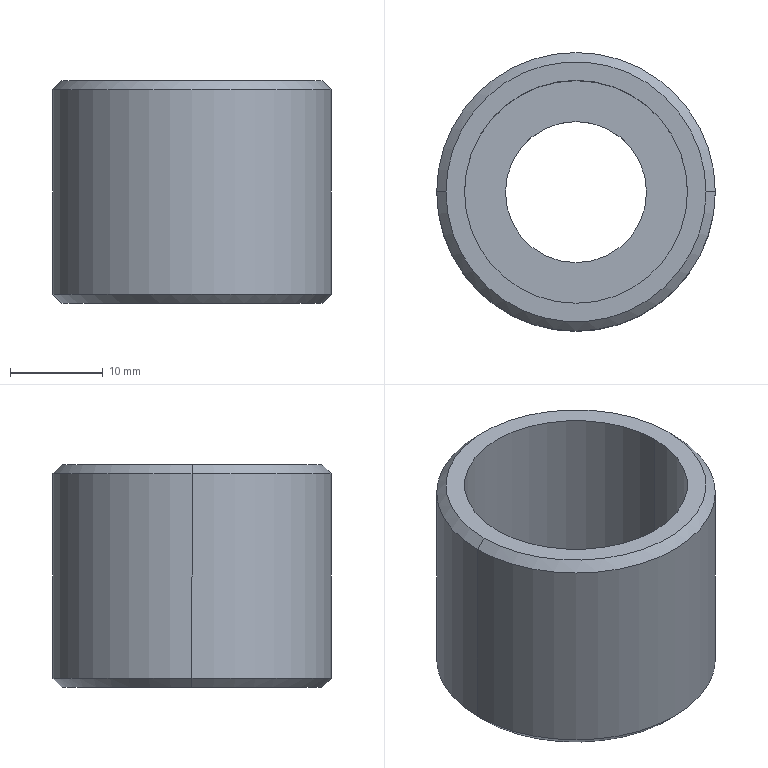Part | STEP file | fBY02F02M-00-16A | 1 solid | 16 faces | box 30 x 30 x 24 mm | volume 7122 mm3 | cylinder 8 | cone 4 | plane 4 | commonest cylinder face diameters 15.2 x2 21 x2 24 x2 30 x2
STEP:
#1=CARTESIAN_POINT('',(0.,0.,0.));
#2=DIRECTION('',(0.,0.,1.));
#3=DIRECTION('',(1.,0.,0.));
#4=AXIS2_PLACEMENT_3D('',#1,#2,#3);
#5=CARTESIAN_POINT('',(-15.,0.,23.));
#6=VERTEX_POINT('',#5);
#7=CARTESIAN_POINT('',(15.,0.,23.));
#8=VERTEX_POINT('',#7);
#9=CARTESIAN_POINT('',(0.,0.,23.));
#10=DIRECTION('',(0.,0.,-1.));
#11=DIRECTION('',(-1.,0.,0.));
#12=AXIS2_PLACEMENT_3D('',#9,#10,#11);
#13=CIRCLE('',#12,15.);
#14=CARTESIAN_POINT('',(0.,0.,24.));
#15=DIRECTION('',(0.,0.,-1.));
#16=DIRECTION('',(-1.,0.,0.));
#17=AXIS2_PLACEMENT_3D('',#14,#15,#16);
#18=CYLINDRICAL_SURFACE('',#17,15.);
#19=CARTESIAN_POINT('',(0.,1.));
#20=DIRECTION('',(1.,0.));
#21=VECTOR('',#20,1.);
#22=LINE('',#19,#21);
#23=(GEOMETRIC_REPRESENTATION_CONTEXT(2)PARAMETRIC_REPRESENTATION_CONTEXT()REPRESENTATION_CONTEXT('',''));
#24=DEFINITIONAL_REPRESENTATION('',(#22),#23);
#25=PCURVE('',#18,#24);
#26=CARTESIAN_POINT('',(0.,0.,23.));
#27=DIRECTION('',(0.,0.,-1.));
#28=DIRECTION('',(-1.,0.,0.));
#29=AXIS2_PLACEMENT_3D('',#26,#27,#28);
#30=CONICAL_SURFACE('',#29,15.,0.7854);
#31=CARTESIAN_POINT('',(0.,0.));
#32=DIRECTION('',(1.,0.));
#33=VECTOR('',#32,1.);
#34=LINE('',#31,#33);
#35=(GEOMETRIC_REPRESENTATION_CONTEXT(2)PARAMETRIC_REPRESENTATION_CONTEXT()REPRESENTATION_CONTEXT('',''));
#36=DEFINITIONAL_REPRESENTATION('',(#34),#35);
#37=PCURVE('',#30,#36);
#38=SURFACE_CURVE('',#13,(#25,#37),.PCURVE_S1.);
#39=EDGE_CURVE('',#6,#8,#38,.T.);
#40=ORIENTED_EDGE('',*,*,#39,.T.);
#41=CARTESIAN_POINT('',(15.,0.,1.));
#42=VERTEX_POINT('',#41);
#43=CARTESIAN_POINT('',(15.,0.,24.));
#44=DIRECTION('',(0.,0.,-1.));
#45=VECTOR('',#44,1.);
#46=LINE('',#43,#45);
#47=CARTESIAN_POINT('',(3.142,0.));
#48=DIRECTION('',(0.,1.));
#49=VECTOR('',#48,1.);
#50=LINE('',#47,#49);
#51=(GEOMETRIC_REPRESENTATION_CONTEXT(2)PARAMETRIC_REPRESENTATION_CONTEXT()REPRESENTATION_CONTEXT('',''));
#52=DEFINITIONAL_REPRESENTATION('',(#50),#51);
#53=PCURVE('',#18,#52);
#54=CARTESIAN_POINT('',(0.,0.,24.));
#55=DIRECTION('',(0.,0.,-1.));
#56=DIRECTION('',(-1.,0.,0.));
#57=AXIS2_PLACEMENT_3D('',#54,#55,#56);
#58=CYLINDRICAL_SURFACE('',#57,15.);
#59=CARTESIAN_POINT('',(3.142,0.));
#60=DIRECTION('',(0.,1.));
#61=VECTOR('',#60,1.);
#62=LINE('',#59,#61);
#63=(GEOMETRIC_REPRESENTATION_CONTEXT(2)PARAMETRIC_REPRESENTATION_CONTEXT()REPRESENTATION_CONTEXT('',''));
#64=DEFINITIONAL_REPRESENTATION('',(#62),#63);
#65=PCURVE('',#58,#64);
#66=SURFACE_CURVE('',#46,(#53,#65),.PCURVE_S1.);
#67=EDGE_CURVE('',#8,#42,#66,.T.);
#68=ORIENTED_EDGE('',*,*,#67,.T.);
#69=CARTESIAN_POINT('',(-15.,0.,1.));
#70=VERTEX_POINT('',#69);
#71=CARTESIAN_POINT('',(0.,0.,1.));
#72=DIRECTION('',(0.,0.,1.));
#73=DIRECTION('',(-1.,0.,0.));
#74=AXIS2_PLACEMENT_3D('',#71,#72,#73);
#75=CIRCLE('',#74,15.);
#76=CARTESIAN_POINT('',(6.283,23.));
#77=DIRECTION('',(-1.,0.));
#78=VECTOR('',#77,1.);
#79=LINE('',#76,#78);
#80=(GEOMETRIC_REPRESENTATION_CONTEXT(2)PARAMETRIC_REPRESENTATION_CONTEXT()REPRESENTATION_CONTEXT('',''));
#81=DEFINITIONAL_REPRESENTATION('',(#79),#80);
#82=PCURVE('',#18,#81);
#83=CARTESIAN_POINT('',(0.,0.,1.));
#84=DIRECTION('',(0.,0.,1.));
#85=DIRECTION('',(1.,0.,0.));
#86=AXIS2_PLACEMENT_3D('',#83,#84,#85);
#87=CONICAL_SURFACE('',#86,15.,0.7854);
#88=CARTESIAN_POINT('',(-3.142,0.));
#89=DIRECTION('',(1.,0.));
#90=VECTOR('',#89,1.);
#91=LINE('',#88,#90);
#92=(GEOMETRIC_REPRESENTATION_CONTEXT(2)PARAMETRIC_REPRESENTATION_CONTEXT()REPRESENTATION_CONTEXT('',''));
#93=DEFINITIONAL_REPRESENTATION('',(#91),#92);
#94=PCURVE('',#87,#93);
#95=SURFACE_CURVE('',#75,(#82,#94),.PCURVE_S1.);
#96=EDGE_CURVE('',#42,#70,#95,.T.);
#97=ORIENTED_EDGE('',*,*,#96,.T.);
#98=CARTESIAN_POINT('',(-15.,0.,24.));
#99=DIRECTION('',(0.,0.,-1.));
#100=VECTOR('',#99,1.);
#101=LINE('',#98,#100);
#102=CARTESIAN_POINT('',(0.,0.));
#103=DIRECTION('',(0.,1.));
#104=VECTOR('',#103,1.);
#105=LINE('',#102,#104);
#106=(GEOMETRIC_REPRESENTATION_CONTEXT(2)PARAMETRIC_REPRESENTATION_CONTEXT()REPRESENTATION_CONTEXT('',''));
#107=DEFINITIONAL_REPRESENTATION('',(#105),#106);
#108=PCURVE('',#18,#107);
#109=CARTESIAN_POINT('',(6.283,0.));
#110=DIRECTION('',(0.,1.));
#111=VECTOR('',#110,1.);
#112=LINE('',#109,#111);
#113=(GEOMETRIC_REPRESENTATION_CONTEXT(2)PARAMETRIC_REPRESENTATION_CONTEXT()REPRESENTATION_CONTEXT('',''));
#114=DEFINITIONAL_REPRESENTATION('',(#112),#113);
#115=PCURVE('',#58,#114);
#116=SURFACE_CURVE('',#101,(#108,#115),.PCURVE_S1.);
#117=EDGE_CURVE('',#6,#70,#116,.T.);
#118=ORIENTED_EDGE('',*,*,#117,.F.);
#119=EDGE_LOOP('',(#40,#68,#97,#118));
#120=FACE_BOUND('',#119,.T.);
#121=ADVANCED_FACE('',(#120),#18,.T.);
#122=CARTESIAN_POINT('',(14.,0.,0.));
#123=VERTEX_POINT('',#122);
#124=CARTESIAN_POINT('',(-14.,0.,0.));
#125=VERTEX_POINT('',#124);
#126=CARTESIAN_POINT('',(0.,0.,0.));
#127=DIRECTION('',(0.,0.,1.));
#128=DIRECTION('',(1.,0.,0.));
#129=AXIS2_PLACEMENT_3D('',#126,#127,#128);
#130=CIRCLE('',#129,14.);
#131=CARTESIAN_POINT('',(0.,-1.));
#132=DIRECTION('',(1.,0.));
#133=VECTOR('',#132,1.);
#134=LINE('',#131,#133);
#135=(GEOMETRIC_REPRESENTATION_CONTEXT(2)PARAMETRIC_REPRESENTATION_CONTEXT()REPRESENTATION_CONTEXT('',''));
#136=DEFINITIONAL_REPRESENTATION('',(#134),#135);
#137=PCURVE('',#87,#136);
#138=CARTESIAN_POINT('',(0.,0.,0.));
#139=DIRECTION('',(0.,0.,1.));
#140=DIRECTION('',(1.,0.,0.));
#141=AXIS2_PLACEMENT_3D('',#138,#139,#140);
#142=PLANE('',#141);
#143=CARTESIAN_POINT('',(0.,0.));
#144=DIRECTION('',(1.,0.));
#145=AXIS2_PLACEMENT_2D('',#143,#144);
#146=CIRCLE('',#145,14.);
#147=(GEOMETRIC_REPRESENTATION_CONTEXT(2)PARAMETRIC_REPRESENTATION_CONTEXT()REPRESENTATION_CONTEXT('',''));
#148=DEFINITIONAL_REPRESENTATION('',(#146),#147);
#149=PCURVE('',#142,#148);
#150=SURFACE_CURVE('',#130,(#137,#149),.PCURVE_S1.);
#151=EDGE_CURVE('',#123,#125,#150,.T.);
#152=ORIENTED_EDGE('',*,*,#151,.T.);
#153=CARTESIAN_POINT('',(-15.,0.,1.));
#154=DIRECTION('',(-0.7071,0.,0.7071));
#155=VECTOR('',#154,1.);
#156=LINE('',#153,#155);
#157=CARTESIAN_POINT('',(3.142,0.));
#158=DIRECTION('',(0.,1.));
#159=VECTOR('',#158,1.);
#160=LINE('',#157,#159);
#161=(GEOMETRIC_REPRESENTATION_CONTEXT(2)PARAMETRIC_REPRESENTATION_CONTEXT()REPRESENTATION_CONTEXT('',''));
#162=DEFINITIONAL_REPRESENTATION('',(#160),#161);
#163=PCURVE('',#87,#162);
#164=CARTESIAN_POINT('',(0.,0.,1.));
#165=DIRECTION('',(0.,0.,1.));
#166=DIRECTION('',(1.,0.,0.));
#167=AXIS2_PLACEMENT_3D('',#164,#165,#166);
#168=CONICAL_SURFACE('',#167,15.,0.7854);
#169=CARTESIAN_POINT('',(3.142,0.));
#170=DIRECTION('',(0.,1.));
#171=VECTOR('',#170,1.);
#172=LINE('',#169,#171);
#173=(GEOMETRIC_REPRESENTATION_CONTEXT(2)PARAMETRIC_REPRESENTATION_CONTEXT()REPRESENTATION_CONTEXT('',''));
#174=DEFINITIONAL_REPRESENTATION('',(#172),#173);
#175=PCURVE('',#168,#174);
#176=SURFACE_CURVE('',#156,(#163,#175),.PCURVE_S1.);
#177=EDGE_CURVE('',#125,#70,#176,.T.);
#178=ORIENTED_EDGE('',*,*,#177,.T.);
#179=ORIENTED_EDGE('',*,*,#96,.F.);
#180=CARTESIAN_POINT('',(15.,0.,1.));
#181=DIRECTION('',(0.7071,0.,0.7071));
#182=VECTOR('',#181,1.);
#183=LINE('',#180,#182);
#184=CARTESIAN_POINT('',(0.,0.));
#185=DIRECTION('',(0.,1.));
#186=VECTOR('',#185,1.);
#187=LINE('',#184,#186);
#188=(GEOMETRIC_REPRESENTATION_CONTEXT(2)PARAMETRIC_REPRESENTATION_CONTEXT()REPRESENTATION_CONTEXT('',''));
#189=DEFINITIONAL_REPRESENTATION('',(#187),#188);
#190=PCURVE('',#87,#189);
#191=CARTESIAN_POINT('',(6.283,0.));
#192=DIRECTION('',(0.,1.));
#193=VECTOR('',#192,1.);
#194=LINE('',#191,#193);
#195=(GEOMETRIC_REPRESENTATION_CONTEXT(2)PARAMETRIC_REPRESENTATION_CONTEXT()REPRESENTATION_CONTEXT('',''));
#196=DEFINITIONAL_REPRESENTATION('',(#194),#195);
#197=PCURVE('',#168,#196);
#198=SURFACE_CURVE('',#183,(#190,#197),.PCURVE_S1.);
#199=EDGE_CURVE('',#123,#42,#198,.T.);
#200=ORIENTED_EDGE('',*,*,#199,.F.);
#201=EDGE_LOOP('',(#152,#178,#179,#200));
#202=FACE_BOUND('',#201,.T.);
#203=ADVANCED_FACE('',(#202),#87,.T.);
#204=CARTESIAN_POINT('',(-14.,0.,24.));
#205=VERTEX_POINT('',#204);
#206=CARTESIAN_POINT('',(14.,0.,24.));
#207=VERTEX_POINT('',#206);
#208=CARTESIAN_POINT('',(0.,0.,24.));
#209=DIRECTION('',(0.,0.,-1.));
#210=DIRECTION('',(-1.,0.,0.));
#211=AXIS2_PLACEMENT_3D('',#208,#209,#210);
#212=CIRCLE('',#211,14.);
#213=CARTESIAN_POINT('',(0.,-1.));
#214=DIRECTION('',(1.,0.));
#215=VECTOR('',#214,1.);
#216=LINE('',#213,#215);
#217=(GEOMETRIC_REPRESENTATION_CONTEXT(2)PARAMETRIC_REPRESENTATION_CONTEXT()REPRESENTATION_CONTEXT('',''));
#218=DEFINITIONAL_REPRESENTATION('',(#216),#217);
#219=PCURVE('',#30,#218);
#220=CARTESIAN_POINT('',(0.,0.,24.));
#221=DIRECTION('',(0.,0.,1.));
#222=DIRECTION('',(1.,0.,0.));
#223=AXIS2_PLACEMENT_3D('',#220,#221,#222);
#224=PLANE('',#223);
#225=CARTESIAN_POINT('',(-14.,0.));
#226=CARTESIAN_POINT('',(-14.,24.249));
#227=CARTESIAN_POINT('',(7.,12.124));
#228=CARTESIAN_POINT('',(28.,0.));
#229=CARTESIAN_POINT('',(7.,-12.124));
#230=CARTESIAN_POINT('',(-14.,-24.249));
#231=CARTESIAN_POINT('',(-14.,0.));
#232=(BOUNDED_CURVE()B_SPLINE_CURVE(2,(#225,#226,#227,#228,#229,#230,#231),.UNSPECIFIED.,.T.,.F.)B_SPLINE_CURVE_WITH_KNOTS((1,2,2,2,2,1),(-2.094,0.,2.094,4.189,6.283,8.378),.UNSPECIFIED.)CURVE()GEOMETRIC_REPRESENTATION_ITEM()RATIONAL_B_SPLINE_CURVE((1.,0.5,1.,0.5,1.,0.5,1.))REPRESENTATION_ITEM(''));
#233=(GEOMETRIC_REPRESENTATION_CONTEXT(2)PARAMETRIC_REPRESENTATION_CONTEXT()REPRESENTATION_CONTEXT('',''));
#234=DEFINITIONAL_REPRESENTATION('',(#232),#233);
#235=PCURVE('',#224,#234);
#236=SURFACE_CURVE('',#212,(#219,#235),.PCURVE_S1.);
#237=EDGE_CURVE('',#205,#207,#236,.T.);
#238=ORIENTED_EDGE('',*,*,#237,.T.);
#239=CARTESIAN_POINT('',(15.,0.,23.));
#240=DIRECTION('',(0.7071,0.,-0.7071));
#241=VECTOR('',#240,1.);
#242=LINE('',#239,#241);
#243=CARTESIAN_POINT('',(3.142,0.));
#244=DIRECTION('',(0.,1.));
#245=VECTOR('',#244,1.);
#246=LINE('',#243,#245);
#247=(GEOMETRIC_REPRESENTATION_CONTEXT(2)PARAMETRIC_REPRESENTATION_CONTEXT()REPRESENTATION_CONTEXT('',''));
#248=DEFINITIONAL_REPRESENTATION('',(#246),#247);
#249=PCURVE('',#30,#248);
#250=CARTESIAN_POINT('',(0.,0.,23.));
#251=DIRECTION('',(0.,0.,-1.));
#252=DIRECTION('',(-1.,0.,0.));
#253=AXIS2_PLACEMENT_3D('',#250,#251,#252);
#254=CONICAL_SURFACE('',#253,15.,0.7854);
#255=CARTESIAN_POINT('',(3.142,0.));
#256=DIRECTION('',(0.,1.));
#257=VECTOR('',#256,1.);
#258=LINE('',#255,#257);
#259=(GEOMETRIC_REPRESENTATION_CONTEXT(2)PARAMETRIC_REPRESENTATION_CONTEXT()REPRESENTATION_CONTEXT('',''));
#260=DEFINITIONAL_REPRESENTATION('',(#258),#259);
#261=PCURVE('',#254,#260);
#262=SURFACE_CURVE('',#242,(#249,#261),.PCURVE_S1.);
#263=EDGE_CURVE('',#207,#8,#262,.T.);
#264=ORIENTED_EDGE('',*,*,#263,.T.);
#265=ORIENTED_EDGE('',*,*,#39,.F.);
#266=CARTESIAN_POINT('',(-15.,0.,23.));
#267=DIRECTION('',(-0.7071,0.,-0.7071));
#268=VECTOR('',#267,1.);
#269=LINE('',#266,#268);
#270=CARTESIAN_POINT('',(0.,0.));
#271=DIRECTION('',(0.,1.));
#272=VECTOR('',#271,1.);
#273=LINE('',#270,#272);
#274=(GEOMETRIC_REPRESENTATION_CONTEXT(2)PARAMETRIC_REPRESENTATION_CONTEXT()REPRESENTATION_CONTEXT('',''));
#275=DEFINITIONAL_REPRESENTATION('',(#273),#274);
#276=PCURVE('',#30,#275);
#277=CARTESIAN_POINT('',(6.283,0.));
#278=DIRECTION('',(0.,1.));
#279=VECTOR('',#278,1.);
#280=LINE('',#277,#279);
#281=(GEOMETRIC_REPRESENTATION_CONTEXT(2)PARAMETRIC_REPRESENTATION_CONTEXT()REPRESENTATION_CONTEXT('',''));
#282=DEFINITIONAL_REPRESENTATION('',(#280),#281);
#283=PCURVE('',#254,#282);
#284=SURFACE_CURVE('',#269,(#276,#283),.PCURVE_S1.);
#285=EDGE_CURVE('',#205,#6,#284,.T.);
#286=ORIENTED_EDGE('',*,*,#285,.F.);
#287=EDGE_LOOP('',(#238,#264,#265,#286));
#288=FACE_BOUND('',#287,.T.);
#289=ADVANCED_FACE('',(#288),#30,.T.);
#290=CARTESIAN_POINT('',(-10.5,0.,1.5));
#291=VERTEX_POINT('',#290);
#292=CARTESIAN_POINT('',(-10.5,0.,0.));
#293=VERTEX_POINT('',#292);
#294=CARTESIAN_POINT('',(-10.5,0.,1.5));
#295=DIRECTION('',(0.,0.,-1.));
#296=VECTOR('',#295,1.);
#297=LINE('',#294,#296);
#298=CARTESIAN_POINT('',(0.,0.,1.5));
#299=DIRECTION('',(0.,0.,-1.));
#300=DIRECTION('',(-1.,0.,0.));
#301=AXIS2_PLACEMENT_3D('',#298,#299,#300);
#302=CYLINDRICAL_SURFACE('',#301,10.5);
#303=CARTESIAN_POINT('',(6.283,0.));
#304=DIRECTION('',(0.,1.));
#305=VECTOR('',#304,1.);
#306=LINE('',#303,#305);
#307=(GEOMETRIC_REPRESENTATION_CONTEXT(2)PARAMETRIC_REPRESENTATION_CONTEXT()REPRESENTATION_CONTEXT('',''));
#308=DEFINITIONAL_REPRESENTATION('',(#306),#307);
#309=PCURVE('',#302,#308);
#310=CARTESIAN_POINT('',(0.,0.,1.5));
#311=DIRECTION('',(0.,0.,-1.));
#312=DIRECTION('',(-1.,0.,0.));
#313=AXIS2_PLACEMENT_3D('',#310,#311,#312);
#314=CYLINDRICAL_SURFACE('',#313,10.5);
#315=CARTESIAN_POINT('',(0.,0.));
#316=DIRECTION('',(0.,1.));
#317=VECTOR('',#316,1.);
#318=LINE('',#315,#317);
#319=(GEOMETRIC_REPRESENTATION_CONTEXT(2)PARAMETRIC_REPRESENTATION_CONTEXT()REPRESENTATION_CONTEXT('',''));
#320=DEFINITIONAL_REPRESENTATION('',(#318),#319);
#321=PCURVE('',#314,#320);
#322=SURFACE_CURVE('',#297,(#309,#321),.PCURVE_S1.);
#323=EDGE_CURVE('',#291,#293,#322,.T.);
#324=ORIENTED_EDGE('',*,*,#323,.T.);
#325=CARTESIAN_POINT('',(10.5,0.,0.));
#326=VERTEX_POINT('',#325);
#327=CARTESIAN_POINT('',(0.,0.,0.));
#328=DIRECTION('',(0.,0.,-1.));
#329=DIRECTION('',(-1.,0.,0.));
#330=AXIS2_PLACEMENT_3D('',#327,#328,#329);
#331=CIRCLE('',#330,10.5);
#332=CARTESIAN_POINT('',(0.,1.5));
#333=DIRECTION('',(1.,0.));
#334=VECTOR('',#333,1.);
#335=LINE('',#332,#334);
#336=(GEOMETRIC_REPRESENTATION_CONTEXT(2)PARAMETRIC_REPRESENTATION_CONTEXT()REPRESENTATION_CONTEXT('',''));
#337=DEFINITIONAL_REPRESENTATION('',(#335),#336);
#338=PCURVE('',#302,#337);
#339=CARTESIAN_POINT('',(-10.5,0.));
#340=CARTESIAN_POINT('',(-10.5,18.187));
#341=CARTESIAN_POINT('',(5.25,9.093));
#342=CARTESIAN_POINT('',(21.,0.));
#343=CARTESIAN_POINT('',(5.25,-9.093));
#344=CARTESIAN_POINT('',(-10.5,-18.187));
#345=CARTESIAN_POINT('',(-10.5,0.));
#346=(BOUNDED_CURVE()B_SPLINE_CURVE(2,(#339,#340,#341,#342,#343,#344,#345),.UNSPECIFIED.,.T.,.F.)B_SPLINE_CURVE_WITH_KNOTS((1,2,2,2,2,1),(-2.094,0.,2.094,4.189,6.283,8.378),.UNSPECIFIED.)CURVE()GEOMETRIC_REPRESENTATION_ITEM()RATIONAL_B_SPLINE_CURVE((1.,0.5,1.,0.5,1.,0.5,1.))REPRESENTATION_ITEM(''));
#347=(GEOMETRIC_REPRESENTATION_CONTEXT(2)PARAMETRIC_REPRESENTATION_CONTEXT()REPRESENTATION_CONTEXT('',''));
#348=DEFINITIONAL_REPRESENTATION('',(#346),#347);
#349=PCURVE('',#142,#348);
#350=SURFACE_CURVE('',#331,(#338,#349),.PCURVE_S1.);
#351=EDGE_CURVE('',#326,#293,#350,.T.);
#352=ORIENTED_EDGE('',*,*,#351,.F.);
#353=CARTESIAN_POINT('',(10.5,0.,1.5));
#354=VERTEX_POINT('',#353);
#355=CARTESIAN_POINT('',(10.5,0.,1.5));
#356=DIRECTION('',(0.,0.,-1.));
#357=VECTOR('',#356,1.);
#358=LINE('',#355,#357);
#359=CARTESIAN_POINT('',(3.142,0.));
#360=DIRECTION('',(0.,1.));
#361=VECTOR('',#360,1.);
#362=LINE('',#359,#361);
#363=(GEOMETRIC_REPRESENTATION_CONTEXT(2)PARAMETRIC_REPRESENTATION_CONTEXT()REPRESENTATION_CONTEXT('',''));
#364=DEFINITIONAL_REPRESENTATION('',(#362),#363);
#365=PCURVE('',#302,#364);
#366=CARTESIAN_POINT('',(3.142,0.));
#367=DIRECTION('',(0.,1.));
#368=VECTOR('',#367,1.);
#369=LINE('',#366,#368);
#370=(GEOMETRIC_REPRESENTATION_CONTEXT(2)PARAMETRIC_REPRESENTATION_CONTEXT()REPRESENTATION_CONTEXT('',''));
#371=DEFINITIONAL_REPRESENTATION('',(#369),#370);
#372=PCURVE('',#314,#371);
#373=SURFACE_CURVE('',#358,(#365,#372),.PCURVE_S1.);
#374=EDGE_CURVE('',#354,#326,#373,.T.);
#375=ORIENTED_EDGE('',*,*,#374,.F.);
#376=CARTESIAN_POINT('',(0.,0.,1.5));
#377=DIRECTION('',(0.,0.,-1.));
#378=DIRECTION('',(-1.,0.,0.));
#379=AXIS2_PLACEMENT_3D('',#376,#377,#378);
#380=CIRCLE('',#379,10.5);
#381=CARTESIAN_POINT('',(0.,0.));
#382=DIRECTION('',(1.,0.));
#383=VECTOR('',#382,1.);
#384=LINE('',#381,#383);
#385=(GEOMETRIC_REPRESENTATION_CONTEXT(2)PARAMETRIC_REPRESENTATION_CONTEXT()REPRESENTATION_CONTEXT('',''));
#386=DEFINITIONAL_REPRESENTATION('',(#384),#385);
#387=PCURVE('',#302,#386);
#388=CARTESIAN_POINT('',(0.,0.,1.5));
#389=DIRECTION('',(0.,0.,-1.));
#390=DIRECTION('',(-1.,0.,0.));
#391=AXIS2_PLACEMENT_3D('',#388,#389,#390);
#392=PLANE('',#391);
#393=CARTESIAN_POINT('',(0.,0.));
#394=DIRECTION('',(1.,0.));
#395=AXIS2_PLACEMENT_2D('',#393,#394);
#396=CIRCLE('',#395,10.5);
#397=(GEOMETRIC_REPRESENTATION_CONTEXT(2)PARAMETRIC_REPRESENTATION_CONTEXT()REPRESENTATION_CONTEXT('',''));
#398=DEFINITIONAL_REPRESENTATION('',(#396),#397);
#399=PCURVE('',#392,#398);
#400=SURFACE_CURVE('',#380,(#387,#399),.PCURVE_S1.);
#401=EDGE_CURVE('',#354,#291,#400,.T.);
#402=ORIENTED_EDGE('',*,*,#401,.T.);
#403=EDGE_LOOP('',(#324,#352,#375,#402));
#404=FACE_BOUND('',#403,.F.);
#405=ADVANCED_FACE('',(#404),#302,.F.);
#406=CARTESIAN_POINT('',(12.,0.,5.));
#407=VERTEX_POINT('',#406);
#408=CARTESIAN_POINT('',(12.,0.,24.));
#409=VERTEX_POINT('',#408);
#410=CARTESIAN_POINT('',(12.,0.,5.));
#411=DIRECTION('',(0.,0.,1.));
#412=VECTOR('',#411,1.);
#413=LINE('',#410,#412);
#414=CARTESIAN_POINT('',(0.,0.,5.));
#415=DIRECTION('',(0.,0.,1.));
#416=DIRECTION('',(1.,0.,0.));
#417=AXIS2_PLACEMENT_3D('',#414,#415,#416);
#418=CYLINDRICAL_SURFACE('',#417,12.);
#419=CARTESIAN_POINT('',(6.283,0.));
#420=DIRECTION('',(0.,1.));
#421=VECTOR('',#420,1.);
#422=LINE('',#419,#421);
#423=(GEOMETRIC_REPRESENTATION_CONTEXT(2)PARAMETRIC_REPRESENTATION_CONTEXT()REPRESENTATION_CONTEXT('',''));
#424=DEFINITIONAL_REPRESENTATION('',(#422),#423);
#425=PCURVE('',#418,#424);
#426=CARTESIAN_POINT('',(0.,0.,5.));
#427=DIRECTION('',(0.,0.,1.));
#428=DIRECTION('',(1.,0.,0.));
#429=AXIS2_PLACEMENT_3D('',#426,#427,#428);
#430=CYLINDRICAL_SURFACE('',#429,12.);
#431=CARTESIAN_POINT('',(0.,0.));
#432=DIRECTION('',(0.,1.));
#433=VECTOR('',#432,1.);
#434=LINE('',#431,#433);
#435=(GEOMETRIC_REPRESENTATION_CONTEXT(2)PARAMETRIC_REPRESENTATION_CONTEXT()REPRESENTATION_CONTEXT('',''));
#436=DEFINITIONAL_REPRESENTATION('',(#434),#435);
#437=PCURVE('',#430,#436);
#438=SURFACE_CURVE('',#413,(#425,#437),.PCURVE_S1.);
#439=EDGE_CURVE('',#407,#409,#438,.T.);
#440=ORIENTED_EDGE('',*,*,#439,.T.);
#441=CARTESIAN_POINT('',(-12.,0.,24.));
#442=VERTEX_POINT('',#441);
#443=CARTESIAN_POINT('',(0.,0.,24.));
#444=DIRECTION('',(0.,0.,-1.));
#445=DIRECTION('',(1.,0.,0.));
#446=AXIS2_PLACEMENT_3D('',#443,#444,#445);
#447=CIRCLE('',#446,12.);
#448=CARTESIAN_POINT('',(6.283,19.));
#449=DIRECTION('',(-1.,0.));
#450=VECTOR('',#449,1.);
#451=LINE('',#448,#450);
#452=(GEOMETRIC_REPRESENTATION_CONTEXT(2)PARAMETRIC_REPRESENTATION_CONTEXT()REPRESENTATION_CONTEXT('',''));
#453=DEFINITIONAL_REPRESENTATION('',(#451),#452);
#454=PCURVE('',#418,#453);
#455=CARTESIAN_POINT('',(12.,0.));
#456=CARTESIAN_POINT('',(12.,-20.785));
#457=CARTESIAN_POINT('',(-6.,-10.392));
#458=CARTESIAN_POINT('',(-24.,0.));
#459=CARTESIAN_POINT('',(-6.,10.392));
#460=CARTESIAN_POINT('',(12.,20.785));
#461=CARTESIAN_POINT('',(12.,0.));
#462=(BOUNDED_CURVE()B_SPLINE_CURVE(2,(#455,#456,#457,#458,#459,#460,#461),.UNSPECIFIED.,.T.,.F.)B_SPLINE_CURVE_WITH_KNOTS((1,2,2,2,2,1),(-2.094,0.,2.094,4.189,6.283,8.378),.UNSPECIFIED.)CURVE()GEOMETRIC_REPRESENTATION_ITEM()RATIONAL_B_SPLINE_CURVE((1.,0.5,1.,0.5,1.,0.5,1.))REPRESENTATION_ITEM(''));
#463=(GEOMETRIC_REPRESENTATION_CONTEXT(2)PARAMETRIC_REPRESENTATION_CONTEXT()REPRESENTATION_CONTEXT('',''));
#464=DEFINITIONAL_REPRESENTATION('',(#462),#463);
#465=PCURVE('',#224,#464);
#466=SURFACE_CURVE('',#447,(#454,#465),.PCURVE_S1.);
#467=EDGE_CURVE('',#409,#442,#466,.T.);
#468=ORIENTED_EDGE('',*,*,#467,.T.);
#469=CARTESIAN_POINT('',(-12.,0.,5.));
#470=VERTEX_POINT('',#469);
#471=CARTESIAN_POINT('',(-12.,0.,5.));
#472=DIRECTION('',(0.,0.,1.));
#473=VECTOR('',#472,1.);
#474=LINE('',#471,#473);
#475=CARTESIAN_POINT('',(3.142,0.));
#476=DIRECTION('',(0.,1.));
#477=VECTOR('',#476,1.);
#478=LINE('',#475,#477);
#479=(GEOMETRIC_REPRESENTATION_CONTEXT(2)PARAMETRIC_REPRESENTATION_CONTEXT()REPRESENTATION_CONTEXT('',''));
#480=DEFINITIONAL_REPRESENTATION('',(#478),#479);
#481=PCURVE('',#418,#480);
#482=CARTESIAN_POINT('',(3.142,0.));
#483=DIRECTION('',(0.,1.));
#484=VECTOR('',#483,1.);
#485=LINE('',#482,#484);
#486=(GEOMETRIC_REPRESENTATION_CONTEXT(2)PARAMETRIC_REPRESENTATION_CONTEXT()REPRESENTATION_CONTEXT('',''));
#487=DEFINITIONAL_REPRESENTATION('',(#485),#486);
#488=PCURVE('',#430,#487);
#489=SURFACE_CURVE('',#474,(#481,#488),.PCURVE_S1.);
#490=EDGE_CURVE('',#470,#442,#489,.T.);
#491=ORIENTED_EDGE('',*,*,#490,.F.);
#492=CARTESIAN_POINT('',(0.,0.,5.));
#493=DIRECTION('',(0.,0.,1.));
#494=DIRECTION('',(1.,0.,0.));
#495=AXIS2_PLACEMENT_3D('',#492,#493,#494);
#496=CIRCLE('',#495,12.);
#497=CARTESIAN_POINT('',(0.,0.));
#498=DIRECTION('',(1.,0.));
#499=VECTOR('',#498,1.);
#500=LINE('',#497,#499);
#501=(GEOMETRIC_REPRESENTATION_CONTEXT(2)PARAMETRIC_REPRESENTATION_CONTEXT()REPRESENTATION_CONTEXT('',''));
#502=DEFINITIONAL_REPRESENTATION('',(#500),#501);
#503=PCURVE('',#418,#502);
#504=CARTESIAN_POINT('',(0.,0.,5.));
#505=DIRECTION('',(0.,0.,1.));
#506=DIRECTION('',(1.,0.,0.));
#507=AXIS2_PLACEMENT_3D('',#504,#505,#506);
#508=PLANE('',#507);
#509=CARTESIAN_POINT('',(0.,0.));
#510=DIRECTION('',(1.,0.));
#511=AXIS2_PLACEMENT_2D('',#509,#510);
#512=CIRCLE('',#511,12.);
#513=(GEOMETRIC_REPRESENTATION_CONTEXT(2)PARAMETRIC_REPRESENTATION_CONTEXT()REPRESENTATION_CONTEXT('',''));
#514=DEFINITIONAL_REPRESENTATION('',(#512),#513);
#515=PCURVE('',#508,#514);
#516=SURFACE_CURVE('',#496,(#503,#515),.PCURVE_S1.);
#517=EDGE_CURVE('',#470,#407,#516,.T.);
#518=ORIENTED_EDGE('',*,*,#517,.T.);
#519=EDGE_LOOP('',(#440,#468,#491,#518));
#520=FACE_BOUND('',#519,.F.);
#521=ADVANCED_FACE('',(#520),#418,.F.);
#522=CARTESIAN_POINT('',(-7.6,0.,5.));
#523=VERTEX_POINT('',#522);
#524=CARTESIAN_POINT('',(-7.6,0.,1.5));
#525=VERTEX_POINT('',#524);
#526=CARTESIAN_POINT('',(-7.6,0.,24.));
#527=DIRECTION('',(0.,0.,-1.));
#528=VECTOR('',#527,1.);
#529=LINE('',#526,#528);
#530=CARTESIAN_POINT('',(0.,0.,24.));
#531=DIRECTION('',(0.,0.,-1.));
#532=DIRECTION('',(-1.,0.,0.));
#533=AXIS2_PLACEMENT_3D('',#530,#531,#532);
#534=CYLINDRICAL_SURFACE('',#533,7.6);
#535=CARTESIAN_POINT('',(6.283,0.));
#536=DIRECTION('',(0.,1.));
#537=VECTOR('',#536,1.);
#538=LINE('',#535,#537);
#539=(GEOMETRIC_REPRESENTATION_CONTEXT(2)PARAMETRIC_REPRESENTATION_CONTEXT()REPRESENTATION_CONTEXT('',''));
#540=DEFINITIONAL_REPRESENTATION('',(#538),#539);
#541=PCURVE('',#534,#540);
#542=CARTESIAN_POINT('',(0.,0.,24.));
#543=DIRECTION('',(0.,0.,-1.));
#544=DIRECTION('',(-1.,0.,0.));
#545=AXIS2_PLACEMENT_3D('',#542,#543,#544);
#546=CYLINDRICAL_SURFACE('',#545,7.6);
#547=CARTESIAN_POINT('',(0.,0.));
#548=DIRECTION('',(0.,1.));
#549=VECTOR('',#548,1.);
#550=LINE('',#547,#549);
#551=(GEOMETRIC_REPRESENTATION_CONTEXT(2)PARAMETRIC_REPRESENTATION_CONTEXT()REPRESENTATION_CONTEXT('',''));
#552=DEFINITIONAL_REPRESENTATION('',(#550),#551);
#553=PCURVE('',#546,#552);
#554=SURFACE_CURVE('',#529,(#541,#553),.PCURVE_S1.);
#555=EDGE_CURVE('',#523,#525,#554,.T.);
#556=ORIENTED_EDGE('',*,*,#555,.T.);
#557=CARTESIAN_POINT('',(7.6,0.,1.5));
#558=VERTEX_POINT('',#557);
#559=CARTESIAN_POINT('',(0.,0.,1.5));
#560=DIRECTION('',(0.,0.,1.));
#561=DIRECTION('',(-1.,0.,0.));
#562=AXIS2_PLACEMENT_3D('',#559,#560,#561);
#563=CIRCLE('',#562,7.6);
#564=CARTESIAN_POINT('',(6.283,22.5));
#565=DIRECTION('',(-1.,0.));
#566=VECTOR('',#565,1.);
#567=LINE('',#564,#566);
#568=(GEOMETRIC_REPRESENTATION_CONTEXT(2)PARAMETRIC_REPRESENTATION_CONTEXT()REPRESENTATION_CONTEXT('',''));
#569=DEFINITIONAL_REPRESENTATION('',(#567),#568);
#570=PCURVE('',#534,#569);
#571=CARTESIAN_POINT('',(7.6,0.));
#572=CARTESIAN_POINT('',(7.6,-13.164));
#573=CARTESIAN_POINT('',(-3.8,-6.582));
#574=CARTESIAN_POINT('',(-15.2,0.));
#575=CARTESIAN_POINT('',(-3.8,6.582));
#576=CARTESIAN_POINT('',(7.6,13.164));
#577=CARTESIAN_POINT('',(7.6,0.));
#578=(BOUNDED_CURVE()B_SPLINE_CURVE(2,(#571,#572,#573,#574,#575,#576,#577),.UNSPECIFIED.,.T.,.F.)B_SPLINE_CURVE_WITH_KNOTS((1,2,2,2,2,1),(-2.094,0.,2.094,4.189,6.283,8.378),.UNSPECIFIED.)CURVE()GEOMETRIC_REPRESENTATION_ITEM()RATIONAL_B_SPLINE_CURVE((1.,0.5,1.,0.5,1.,0.5,1.))REPRESENTATION_ITEM(''));
#579=(GEOMETRIC_REPRESENTATION_CONTEXT(2)PARAMETRIC_REPRESENTATION_CONTEXT()REPRESENTATION_CONTEXT('',''));
#580=DEFINITIONAL_REPRESENTATION('',(#578),#579);
#581=PCURVE('',#392,#580);
#582=SURFACE_CURVE('',#563,(#570,#581),.PCURVE_S1.);
#583=EDGE_CURVE('',#525,#558,#582,.T.);
#584=ORIENTED_EDGE('',*,*,#583,.T.);
#585=CARTESIAN_POINT('',(7.6,0.,5.));
#586=VERTEX_POINT('',#585);
#587=CARTESIAN_POINT('',(7.6,0.,24.));
#588=DIRECTION('',(0.,0.,-1.));
#589=VECTOR('',#588,1.);
#590=LINE('',#587,#589);
#591=CARTESIAN_POINT('',(3.142,0.));
#592=DIRECTION('',(0.,1.));
#593=VECTOR('',#592,1.);
#594=LINE('',#591,#593);
#595=(GEOMETRIC_REPRESENTATION_CONTEXT(2)PARAMETRIC_REPRESENTATION_CONTEXT()REPRESENTATION_CONTEXT('',''));
#596=DEFINITIONAL_REPRESENTATION('',(#594),#595);
#597=PCURVE('',#534,#596);
#598=CARTESIAN_POINT('',(3.142,0.));
#599=DIRECTION('',(0.,1.));
#600=VECTOR('',#599,1.);
#601=LINE('',#598,#600);
#602=(GEOMETRIC_REPRESENTATION_CONTEXT(2)PARAMETRIC_REPRESENTATION_CONTEXT()REPRESENTATION_CONTEXT('',''));
#603=DEFINITIONAL_REPRESENTATION('',(#601),#602);
#604=PCURVE('',#546,#603);
#605=SURFACE_CURVE('',#590,(#597,#604),.PCURVE_S1.);
#606=EDGE_CURVE('',#586,#558,#605,.T.);
#607=ORIENTED_EDGE('',*,*,#606,.F.);
#608=CARTESIAN_POINT('',(0.,0.,5.));
#609=DIRECTION('',(0.,0.,-1.));
#610=DIRECTION('',(-1.,0.,0.));
#611=AXIS2_PLACEMENT_3D('',#608,#609,#610);
#612=CIRCLE('',#611,7.6);
#613=CARTESIAN_POINT('',(0.,19.));
#614=DIRECTION('',(1.,0.));
#615=VECTOR('',#614,1.);
#616=LINE('',#613,#615);
#617=(GEOMETRIC_REPRESENTATION_CONTEXT(2)PARAMETRIC_REPRESENTATION_CONTEXT()REPRESENTATION_CONTEXT('',''));
#618=DEFINITIONAL_REPRESENTATION('',(#616),#617);
#619=PCURVE('',#534,#618);
#620=CARTESIAN_POINT('',(-7.6,0.));
#621=CARTESIAN_POINT('',(-7.6,13.164));
#622=CARTESIAN_POINT('',(3.8,6.582));
#623=CARTESIAN_POINT('',(15.2,0.));
#624=CARTESIAN_POINT('',(3.8,-6.582));
#625=CARTESIAN_POINT('',(-7.6,-13.164));
#626=CARTESIAN_POINT('',(-7.6,0.));
#627=(BOUNDED_CURVE()B_SPLINE_CURVE(2,(#620,#621,#622,#623,#624,#625,#626),.UNSPECIFIED.,.T.,.F.)B_SPLINE_CURVE_WITH_KNOTS((1,2,2,2,2,1),(-2.094,0.,2.094,4.189,6.283,8.378),.UNSPECIFIED.)CURVE()GEOMETRIC_REPRESENTATION_ITEM()RATIONAL_B_SPLINE_CURVE((1.,0.5,1.,0.5,1.,0.5,1.))REPRESENTATION_ITEM(''));
#628=(GEOMETRIC_REPRESENTATION_CONTEXT(2)PARAMETRIC_REPRESENTATION_CONTEXT()REPRESENTATION_CONTEXT('',''));
#629=DEFINITIONAL_REPRESENTATION('',(#627),#628);
#630=PCURVE('',#508,#629);
#631=SURFACE_CURVE('',#612,(#619,#630),.PCURVE_S1.);
#632=EDGE_CURVE('',#586,#523,#631,.T.);
#633=ORIENTED_EDGE('',*,*,#632,.T.);
#634=EDGE_LOOP('',(#556,#584,#607,#633));
#635=FACE_BOUND('',#634,.F.);
#636=ADVANCED_FACE('',(#635),#534,.F.);
#637=ORIENTED_EDGE('',*,*,#67,.F.);
#638=CARTESIAN_POINT('',(0.,0.,23.));
#639=DIRECTION('',(0.,0.,-1.));
#640=DIRECTION('',(-1.,0.,0.));
#641=AXIS2_PLACEMENT_3D('',#638,#639,#640);
#642=CIRCLE('',#641,15.);
#643=CARTESIAN_POINT('',(0.,1.));
#644=DIRECTION('',(1.,0.));
#645=VECTOR('',#644,1.);
#646=LINE('',#643,#645);
#647=(GEOMETRIC_REPRESENTATION_CONTEXT(2)PARAMETRIC_REPRESENTATION_CONTEXT()REPRESENTATION_CONTEXT('',''));
#648=DEFINITIONAL_REPRESENTATION('',(#646),#647);
#649=PCURVE('',#58,#648);
#650=CARTESIAN_POINT('',(0.,0.));
#651=DIRECTION('',(1.,0.));
#652=VECTOR('',#651,1.);
#653=LINE('',#650,#652);
#654=(GEOMETRIC_REPRESENTATION_CONTEXT(2)PARAMETRIC_REPRESENTATION_CONTEXT()REPRESENTATION_CONTEXT('',''));
#655=DEFINITIONAL_REPRESENTATION('',(#653),#654);
#656=PCURVE('',#254,#655);
#657=SURFACE_CURVE('',#642,(#649,#656),.PCURVE_S1.);
#658=EDGE_CURVE('',#8,#6,#657,.T.);
#659=ORIENTED_EDGE('',*,*,#658,.T.);
#660=ORIENTED_EDGE('',*,*,#117,.T.);
#661=CARTESIAN_POINT('',(0.,0.,1.));
#662=DIRECTION('',(0.,0.,1.));
#663=DIRECTION('',(-1.,0.,0.));
#664=AXIS2_PLACEMENT_3D('',#661,#662,#663);
#665=CIRCLE('',#664,15.);
#666=CARTESIAN_POINT('',(6.283,23.));
#667=DIRECTION('',(-1.,0.));
#668=VECTOR('',#667,1.);
#669=LINE('',#666,#668);
#670=(GEOMETRIC_REPRESENTATION_CONTEXT(2)PARAMETRIC_REPRESENTATION_CONTEXT()REPRESENTATION_CONTEXT('',''));
#671=DEFINITIONAL_REPRESENTATION('',(#669),#670);
#672=PCURVE('',#58,#671);
#673=CARTESIAN_POINT('',(3.142,0.));
#674=DIRECTION('',(1.,0.));
#675=VECTOR('',#674,1.);
#676=LINE('',#673,#675);
#677=(GEOMETRIC_REPRESENTATION_CONTEXT(2)PARAMETRIC_REPRESENTATION_CONTEXT()REPRESENTATION_CONTEXT('',''));
#678=DEFINITIONAL_REPRESENTATION('',(#676),#677);
#679=PCURVE('',#168,#678);
#680=SURFACE_CURVE('',#665,(#672,#679),.PCURVE_S1.);
#681=EDGE_CURVE('',#70,#42,#680,.T.);
#682=ORIENTED_EDGE('',*,*,#681,.T.);
#683=EDGE_LOOP('',(#637,#659,#660,#682));
#684=FACE_BOUND('',#683,.T.);
#685=ADVANCED_FACE('',(#684),#58,.T.);
#686=ORIENTED_EDGE('',*,*,#177,.F.);
#687=CARTESIAN_POINT('',(0.,0.,0.));
#688=DIRECTION('',(0.,0.,1.));
#689=DIRECTION('',(1.,0.,0.));
#690=AXIS2_PLACEMENT_3D('',#687,#688,#689);
#691=CIRCLE('',#690,14.);
#692=CARTESIAN_POINT('',(0.,-1.));
#693=DIRECTION('',(1.,0.));
#694=VECTOR('',#693,1.);
#695=LINE('',#692,#694);
#696=(GEOMETRIC_REPRESENTATION_CONTEXT(2)PARAMETRIC_REPRESENTATION_CONTEXT()REPRESENTATION_CONTEXT('',''));
#697=DEFINITIONAL_REPRESENTATION('',(#695),#696);
#698=PCURVE('',#168,#697);
#699=CARTESIAN_POINT('',(0.,0.));
#700=DIRECTION('',(1.,0.));
#701=AXIS2_PLACEMENT_2D('',#699,#700);
#702=CIRCLE('',#701,14.);
#703=(GEOMETRIC_REPRESENTATION_CONTEXT(2)PARAMETRIC_REPRESENTATION_CONTEXT()REPRESENTATION_CONTEXT('',''));
#704=DEFINITIONAL_REPRESENTATION('',(#702),#703);
#705=PCURVE('',#142,#704);
#706=SURFACE_CURVE('',#691,(#698,#705),.PCURVE_S1.);
#707=EDGE_CURVE('',#125,#123,#706,.T.);
#708=ORIENTED_EDGE('',*,*,#707,.T.);
#709=ORIENTED_EDGE('',*,*,#199,.T.);
#710=ORIENTED_EDGE('',*,*,#681,.F.);
#711=EDGE_LOOP('',(#686,#708,#709,#710));
#712=FACE_BOUND('',#711,.T.);
#713=ADVANCED_FACE('',(#712),#168,.T.);
#714=ORIENTED_EDGE('',*,*,#263,.F.);
#715=CARTESIAN_POINT('',(0.,0.,24.));
#716=DIRECTION('',(0.,0.,-1.));
#717=DIRECTION('',(-1.,0.,0.));
#718=AXIS2_PLACEMENT_3D('',#715,#716,#717);
#719=CIRCLE('',#718,14.);
#720=CARTESIAN_POINT('',(0.,-1.));
#721=DIRECTION('',(1.,0.));
#722=VECTOR('',#721,1.);
#723=LINE('',#720,#722);
#724=(GEOMETRIC_REPRESENTATION_CONTEXT(2)PARAMETRIC_REPRESENTATION_CONTEXT()REPRESENTATION_CONTEXT('',''));
#725=DEFINITIONAL_REPRESENTATION('',(#723),#724);
#726=PCURVE('',#254,#725);
#727=CARTESIAN_POINT('',(-14.,0.));
#728=CARTESIAN_POINT('',(-14.,24.249));
#729=CARTESIAN_POINT('',(7.,12.124));
#730=CARTESIAN_POINT('',(28.,0.));
#731=CARTESIAN_POINT('',(7.,-12.124));
#732=CARTESIAN_POINT('',(-14.,-24.249));
#733=CARTESIAN_POINT('',(-14.,0.));
#734=(BOUNDED_CURVE()B_SPLINE_CURVE(2,(#727,#728,#729,#730,#731,#732,#733),.UNSPECIFIED.,.T.,.F.)B_SPLINE_CURVE_WITH_KNOTS((1,2,2,2,2,1),(-2.094,0.,2.094,4.189,6.283,8.378),.UNSPECIFIED.)CURVE()GEOMETRIC_REPRESENTATION_ITEM()RATIONAL_B_SPLINE_CURVE((1.,0.5,1.,0.5,1.,0.5,1.))REPRESENTATION_ITEM(''));
#735=(GEOMETRIC_REPRESENTATION_CONTEXT(2)PARAMETRIC_REPRESENTATION_CONTEXT()REPRESENTATION_CONTEXT('',''));
#736=DEFINITIONAL_REPRESENTATION('',(#734),#735);
#737=PCURVE('',#224,#736);
#738=SURFACE_CURVE('',#719,(#726,#737),.PCURVE_S1.);
#739=EDGE_CURVE('',#207,#205,#738,.T.);
#740=ORIENTED_EDGE('',*,*,#739,.T.);
#741=ORIENTED_EDGE('',*,*,#285,.T.);
#742=ORIENTED_EDGE('',*,*,#658,.F.);
#743=EDGE_LOOP('',(#714,#740,#741,#742));
#744=FACE_BOUND('',#743,.T.);
#745=ADVANCED_FACE('',(#744),#254,.T.);
#746=CARTESIAN_POINT('',(0.,0.,0.));
#747=DIRECTION('',(0.,0.,-1.));
#748=DIRECTION('',(-1.,0.,0.));
#749=AXIS2_PLACEMENT_3D('',#746,#747,#748);
#750=CIRCLE('',#749,10.5);
#751=CARTESIAN_POINT('',(-10.5,0.));
#752=CARTESIAN_POINT('',(-10.5,18.187));
#753=CARTESIAN_POINT('',(5.25,9.093));
#754=CARTESIAN_POINT('',(21.,0.));
#755=CARTESIAN_POINT('',(5.25,-9.093));
#756=CARTESIAN_POINT('',(-10.5,-18.187));
#757=CARTESIAN_POINT('',(-10.5,0.));
#758=(BOUNDED_CURVE()B_SPLINE_CURVE(2,(#751,#752,#753,#754,#755,#756,#757),.UNSPECIFIED.,.T.,.F.)B_SPLINE_CURVE_WITH_KNOTS((1,2,2,2,2,1),(-2.094,0.,2.094,4.189,6.283,8.378),.UNSPECIFIED.)CURVE()GEOMETRIC_REPRESENTATION_ITEM()RATIONAL_B_SPLINE_CURVE((1.,0.5,1.,0.5,1.,0.5,1.))REPRESENTATION_ITEM(''));
#759=(GEOMETRIC_REPRESENTATION_CONTEXT(2)PARAMETRIC_REPRESENTATION_CONTEXT()REPRESENTATION_CONTEXT('',''));
#760=DEFINITIONAL_REPRESENTATION('',(#758),#759);
#761=PCURVE('',#142,#760);
#762=CARTESIAN_POINT('',(0.,1.5));
#763=DIRECTION('',(1.,0.));
#764=VECTOR('',#763,1.);
#765=LINE('',#762,#764);
#766=(GEOMETRIC_REPRESENTATION_CONTEXT(2)PARAMETRIC_REPRESENTATION_CONTEXT()REPRESENTATION_CONTEXT('',''));
#767=DEFINITIONAL_REPRESENTATION('',(#765),#766);
#768=PCURVE('',#314,#767);
#769=SURFACE_CURVE('',#750,(#761,#768),.PCURVE_S1.);
#770=EDGE_CURVE('',#293,#326,#769,.T.);
#771=ORIENTED_EDGE('',*,*,#770,.F.);
#772=ORIENTED_EDGE('',*,*,#351,.F.);
#773=EDGE_LOOP('',(#771,#772));
#774=FACE_BOUND('',#773,.T.);
#775=ORIENTED_EDGE('',*,*,#151,.F.);
#776=ORIENTED_EDGE('',*,*,#707,.F.);
#777=EDGE_LOOP('',(#775,#776));
#778=FACE_BOUND('',#777,.T.);
#779=ADVANCED_FACE('',(#774,#778),#142,.F.);
#780=ORIENTED_EDGE('',*,*,#467,.T.);
#781=CARTESIAN_POINT('',(0.,0.,24.));
#782=DIRECTION('',(0.,0.,-1.));
#783=DIRECTION('',(1.,0.,0.));
#784=AXIS2_PLACEMENT_3D('',#781,#782,#783);
#785=CIRCLE('',#784,12.);
#786=CARTESIAN_POINT('',(12.,0.));
#787=CARTESIAN_POINT('',(12.,-20.785));
#788=CARTESIAN_POINT('',(-6.,-10.392));
#789=CARTESIAN_POINT('',(-24.,0.));
#790=CARTESIAN_POINT('',(-6.,10.392));
#791=CARTESIAN_POINT('',(12.,20.785));
#792=CARTESIAN_POINT('',(12.,0.));
#793=(BOUNDED_CURVE()B_SPLINE_CURVE(2,(#786,#787,#788,#789,#790,#791,#792),.UNSPECIFIED.,.T.,.F.)B_SPLINE_CURVE_WITH_KNOTS((1,2,2,2,2,1),(-2.094,0.,2.094,4.189,6.283,8.378),.UNSPECIFIED.)CURVE()GEOMETRIC_REPRESENTATION_ITEM()RATIONAL_B_SPLINE_CURVE((1.,0.5,1.,0.5,1.,0.5,1.))REPRESENTATION_ITEM(''));
#794=(GEOMETRIC_REPRESENTATION_CONTEXT(2)PARAMETRIC_REPRESENTATION_CONTEXT()REPRESENTATION_CONTEXT('',''));
#795=DEFINITIONAL_REPRESENTATION('',(#793),#794);
#796=PCURVE('',#224,#795);
#797=CARTESIAN_POINT('',(6.283,19.));
#798=DIRECTION('',(-1.,0.));
#799=VECTOR('',#798,1.);
#800=LINE('',#797,#799);
#801=(GEOMETRIC_REPRESENTATION_CONTEXT(2)PARAMETRIC_REPRESENTATION_CONTEXT()REPRESENTATION_CONTEXT('',''));
#802=DEFINITIONAL_REPRESENTATION('',(#800),#801);
#803=PCURVE('',#430,#802);
#804=SURFACE_CURVE('',#785,(#796,#803),.PCURVE_S1.);
#805=EDGE_CURVE('',#442,#409,#804,.T.);
#806=ORIENTED_EDGE('',*,*,#805,.T.);
#807=EDGE_LOOP('',(#780,#806));
#808=FACE_BOUND('',#807,.T.);
#809=ORIENTED_EDGE('',*,*,#237,.F.);
#810=ORIENTED_EDGE('',*,*,#739,.F.);
#811=EDGE_LOOP('',(#809,#810));
#812=FACE_BOUND('',#811,.T.);
#813=ADVANCED_FACE('',(#808,#812),#224,.T.);
#814=ORIENTED_EDGE('',*,*,#770,.F.);
#815=ORIENTED_EDGE('',*,*,#323,.F.);
#816=CARTESIAN_POINT('',(0.,0.,1.5));
#817=DIRECTION('',(0.,0.,-1.));
#818=DIRECTION('',(-1.,0.,0.));
#819=AXIS2_PLACEMENT_3D('',#816,#817,#818);
#820=CIRCLE('',#819,10.5);
#821=CARTESIAN_POINT('',(0.,0.));
#822=DIRECTION('',(1.,0.));
#823=VECTOR('',#822,1.);
#824=LINE('',#821,#823);
#825=(GEOMETRIC_REPRESENTATION_CONTEXT(2)PARAMETRIC_REPRESENTATION_CONTEXT()REPRESENTATION_CONTEXT('',''));
#826=DEFINITIONAL_REPRESENTATION('',(#824),#825);
#827=PCURVE('',#314,#826);
#828=CARTESIAN_POINT('',(0.,0.));
#829=DIRECTION('',(1.,0.));
#830=AXIS2_PLACEMENT_2D('',#828,#829);
#831=CIRCLE('',#830,10.5);
#832=(GEOMETRIC_REPRESENTATION_CONTEXT(2)PARAMETRIC_REPRESENTATION_CONTEXT()REPRESENTATION_CONTEXT('',''));
#833=DEFINITIONAL_REPRESENTATION('',(#831),#832);
#834=PCURVE('',#392,#833);
#835=SURFACE_CURVE('',#820,(#827,#834),.PCURVE_S1.);
#836=EDGE_CURVE('',#291,#354,#835,.T.);
#837=ORIENTED_EDGE('',*,*,#836,.T.);
#838=ORIENTED_EDGE('',*,*,#374,.T.);
#839=EDGE_LOOP('',(#814,#815,#837,#838));
#840=FACE_BOUND('',#839,.F.);
#841=ADVANCED_FACE('',(#840),#314,.F.);
#842=ORIENTED_EDGE('',*,*,#805,.T.);
#843=ORIENTED_EDGE('',*,*,#439,.F.);
#844=CARTESIAN_POINT('',(0.,0.,5.));
#845=DIRECTION('',(0.,0.,1.));
#846=DIRECTION('',(1.,0.,0.));
#847=AXIS2_PLACEMENT_3D('',#844,#845,#846);
#848=CIRCLE('',#847,12.);
#849=CARTESIAN_POINT('',(0.,0.));
#850=DIRECTION('',(1.,0.));
#851=VECTOR('',#850,1.);
#852=LINE('',#849,#851);
#853=(GEOMETRIC_REPRESENTATION_CONTEXT(2)PARAMETRIC_REPRESENTATION_CONTEXT()REPRESENTATION_CONTEXT('',''));
#854=DEFINITIONAL_REPRESENTATION('',(#852),#853);
#855=PCURVE('',#430,#854);
#856=CARTESIAN_POINT('',(0.,0.));
#857=DIRECTION('',(1.,0.));
#858=AXIS2_PLACEMENT_2D('',#856,#857);
#859=CIRCLE('',#858,12.);
#860=(GEOMETRIC_REPRESENTATION_CONTEXT(2)PARAMETRIC_REPRESENTATION_CONTEXT()REPRESENTATION_CONTEXT('',''));
#861=DEFINITIONAL_REPRESENTATION('',(#859),#860);
#862=PCURVE('',#508,#861);
#863=SURFACE_CURVE('',#848,(#855,#862),.PCURVE_S1.);
#864=EDGE_CURVE('',#407,#470,#863,.T.);
#865=ORIENTED_EDGE('',*,*,#864,.T.);
#866=ORIENTED_EDGE('',*,*,#490,.T.);
#867=EDGE_LOOP('',(#842,#843,#865,#866));
#868=FACE_BOUND('',#867,.F.);
#869=ADVANCED_FACE('',(#868),#430,.F.);
#870=ORIENTED_EDGE('',*,*,#836,.T.);
#871=ORIENTED_EDGE('',*,*,#401,.T.);
#872=EDGE_LOOP('',(#870,#871));
#873=FACE_BOUND('',#872,.T.);
#874=ORIENTED_EDGE('',*,*,#583,.T.);
#875=CARTESIAN_POINT('',(0.,0.,1.5));
#876=DIRECTION('',(0.,0.,1.));
#877=DIRECTION('',(-1.,0.,0.));
#878=AXIS2_PLACEMENT_3D('',#875,#876,#877);
#879=CIRCLE('',#878,7.6);
#880=CARTESIAN_POINT('',(7.6,0.));
#881=CARTESIAN_POINT('',(7.6,-13.164));
#882=CARTESIAN_POINT('',(-3.8,-6.582));
#883=CARTESIAN_POINT('',(-15.2,0.));
#884=CARTESIAN_POINT('',(-3.8,6.582));
#885=CARTESIAN_POINT('',(7.6,13.164));
#886=CARTESIAN_POINT('',(7.6,0.));
#887=(BOUNDED_CURVE()B_SPLINE_CURVE(2,(#880,#881,#882,#883,#884,#885,#886),.UNSPECIFIED.,.T.,.F.)B_SPLINE_CURVE_WITH_KNOTS((1,2,2,2,2,1),(-2.094,0.,2.094,4.189,6.283,8.378),.UNSPECIFIED.)CURVE()GEOMETRIC_REPRESENTATION_ITEM()RATIONAL_B_SPLINE_CURVE((1.,0.5,1.,0.5,1.,0.5,1.))REPRESENTATION_ITEM(''));
#888=(GEOMETRIC_REPRESENTATION_CONTEXT(2)PARAMETRIC_REPRESENTATION_CONTEXT()REPRESENTATION_CONTEXT('',''));
#889=DEFINITIONAL_REPRESENTATION('',(#887),#888);
#890=PCURVE('',#392,#889);
#891=CARTESIAN_POINT('',(6.283,22.5));
#892=DIRECTION('',(-1.,0.));
#893=VECTOR('',#892,1.);
#894=LINE('',#891,#893);
#895=(GEOMETRIC_REPRESENTATION_CONTEXT(2)PARAMETRIC_REPRESENTATION_CONTEXT()REPRESENTATION_CONTEXT('',''));
#896=DEFINITIONAL_REPRESENTATION('',(#894),#895);
#897=PCURVE('',#546,#896);
#898=SURFACE_CURVE('',#879,(#890,#897),.PCURVE_S1.);
#899=EDGE_CURVE('',#558,#525,#898,.T.);
#900=ORIENTED_EDGE('',*,*,#899,.T.);
#901=EDGE_LOOP('',(#874,#900));
#902=FACE_BOUND('',#901,.T.);
#903=ADVANCED_FACE('',(#873,#902),#392,.T.);
#904=ORIENTED_EDGE('',*,*,#864,.T.);
#905=ORIENTED_EDGE('',*,*,#517,.T.);
#906=EDGE_LOOP('',(#904,#905));
#907=FACE_BOUND('',#906,.T.);
#908=CARTESIAN_POINT('',(0.,0.,5.));
#909=DIRECTION('',(0.,0.,-1.));
#910=DIRECTION('',(-1.,0.,0.));
#911=AXIS2_PLACEMENT_3D('',#908,#909,#910);
#912=CIRCLE('',#911,7.6);
#913=CARTESIAN_POINT('',(-7.6,0.));
#914=CARTESIAN_POINT('',(-7.6,13.164));
#915=CARTESIAN_POINT('',(3.8,6.582));
#916=CARTESIAN_POINT('',(15.2,0.));
#917=CARTESIAN_POINT('',(3.8,-6.582));
#918=CARTESIAN_POINT('',(-7.6,-13.164));
#919=CARTESIAN_POINT('',(-7.6,0.));
#920=(BOUNDED_CURVE()B_SPLINE_CURVE(2,(#913,#914,#915,#916,#917,#918,#919),.UNSPECIFIED.,.T.,.F.)B_SPLINE_CURVE_WITH_KNOTS((1,2,2,2,2,1),(-2.094,0.,2.094,4.189,6.283,8.378),.UNSPECIFIED.)CURVE()GEOMETRIC_REPRESENTATION_ITEM()RATIONAL_B_SPLINE_CURVE((1.,0.5,1.,0.5,1.,0.5,1.))REPRESENTATION_ITEM(''));
#921=(GEOMETRIC_REPRESENTATION_CONTEXT(2)PARAMETRIC_REPRESENTATION_CONTEXT()REPRESENTATION_CONTEXT('',''));
#922=DEFINITIONAL_REPRESENTATION('',(#920),#921);
#923=PCURVE('',#508,#922);
#924=CARTESIAN_POINT('',(0.,19.));
#925=DIRECTION('',(1.,0.));
#926=VECTOR('',#925,1.);
#927=LINE('',#924,#926);
#928=(GEOMETRIC_REPRESENTATION_CONTEXT(2)PARAMETRIC_REPRESENTATION_CONTEXT()REPRESENTATION_CONTEXT('',''));
#929=DEFINITIONAL_REPRESENTATION('',(#927),#928);
#930=PCURVE('',#546,#929);
#931=SURFACE_CURVE('',#912,(#923,#930),.PCURVE_S1.);
#932=EDGE_CURVE('',#523,#586,#931,.T.);
#933=ORIENTED_EDGE('',*,*,#932,.T.);
#934=ORIENTED_EDGE('',*,*,#632,.T.);
#935=EDGE_LOOP('',(#933,#934));
#936=FACE_BOUND('',#935,.T.);
#937=ADVANCED_FACE('',(#907,#936),#508,.T.);
#938=ORIENTED_EDGE('',*,*,#899,.T.);
#939=ORIENTED_EDGE('',*,*,#555,.F.);
#940=ORIENTED_EDGE('',*,*,#932,.T.);
#941=ORIENTED_EDGE('',*,*,#606,.T.);
#942=EDGE_LOOP('',(#938,#939,#940,#941));
#943=FACE_BOUND('',#942,.F.);
#944=ADVANCED_FACE('',(#943),#546,.F.);
#945=CLOSED_SHELL('',(#121,#203,#289,#405,#521,#636,#685,#713,#745,#779,#813,#841,#869,#903,#937,#944));
#946=MANIFOLD_SOLID_BREP('',#945);
#947=(LENGTH_UNIT()NAMED_UNIT(*)SI_UNIT(.MILLI.,.METRE.));
#948=UNCERTAINTY_MEASURE_WITH_UNIT(LENGTH_MEASURE(0.0000001),#947,'','');
#949=(NAMED_UNIT(*)PLANE_ANGLE_UNIT()SI_UNIT($,.RADIAN.));
#950=(NAMED_UNIT(*)SI_UNIT($,.STERADIAN.)SOLID_ANGLE_UNIT());
#951=(GEOMETRIC_REPRESENTATION_CONTEXT(3)GLOBAL_UNCERTAINTY_ASSIGNED_CONTEXT((#948))GLOBAL_UNIT_ASSIGNED_CONTEXT((#947,#949,#950))REPRESENTATION_CONTEXT('',''));
#952=ADVANCED_BREP_SHAPE_REPRESENTATION('',(#4,#946),#951);